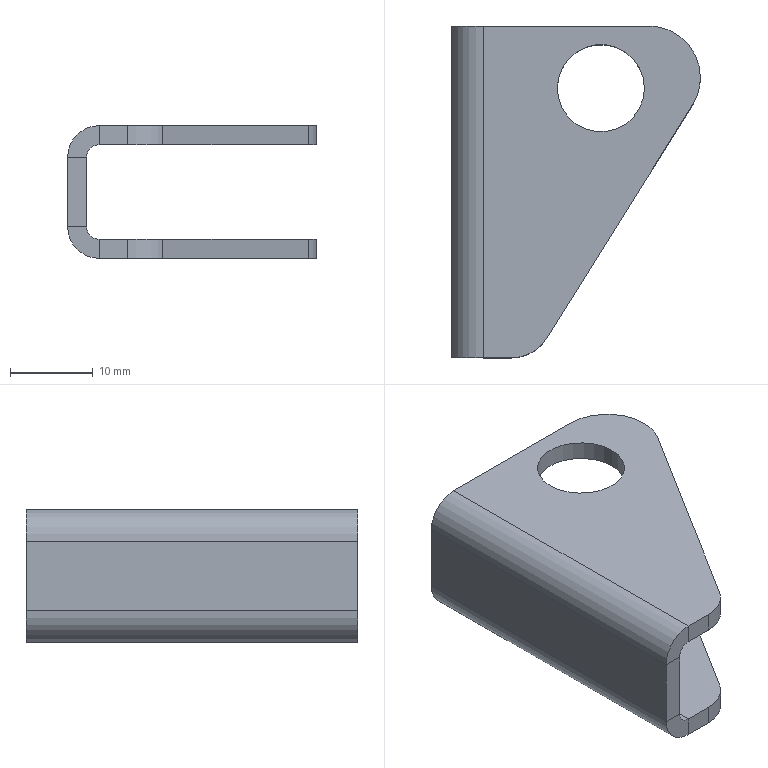Part | STEP file | Input 45 | 1 solid | 32 faces | box 30 x 40 x 16 mm | volume 4444 mm3 | plane 18 | cylinder 14 | commonest cylinder face diameters 10.5 x4 12.434 x4 3 x2 7.6 x2 10 x2